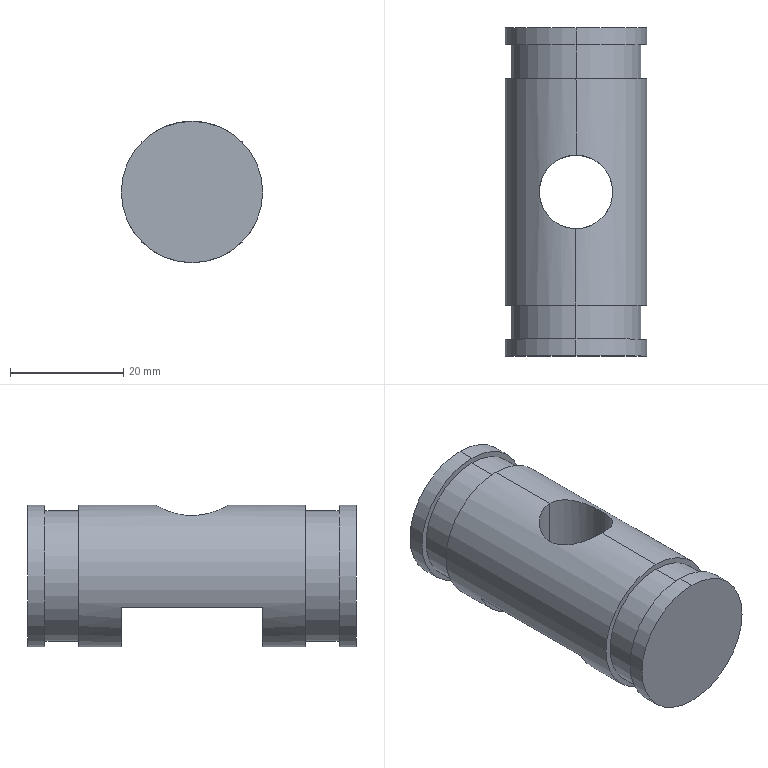Part | SolidWorks | features ICE 3, Extrusion 1, MirrorPattern 1 | 1 solid | 21 faces | box 25 x 58 x 25 mm | volume 22422 mm3 | cylinder 12 | plane 9 | commonest cylinder face diameters 25 x6 23 x4 13 x2
STEP:
#1=CARTESIAN_POINT('',(0.,-6.5,12.5));
#2=VERTEX_POINT('',#1);
#3=CARTESIAN_POINT('',(0.,6.5,12.5));
#4=VERTEX_POINT('',#3);
#5=CARTESIAN_POINT('',(0.,-6.5,12.5));
#6=CARTESIAN_POINT('',(-0.4318,-6.5,12.5));
#7=CARTESIAN_POINT('',(-0.8709,-6.456,12.477));
#8=CARTESIAN_POINT('',(-1.714,-6.285,12.389));
#9=CARTESIAN_POINT('',(-2.124,-6.158,12.325));
#10=CARTESIAN_POINT('',(-2.915,-5.826,12.162));
#11=CARTESIAN_POINT('',(-3.286,-5.624,12.066));
#12=CARTESIAN_POINT('',(-3.982,-5.155,11.854));
#13=CARTESIAN_POINT('',(-4.309,-4.884,11.738));
#14=CARTESIAN_POINT('',(-4.897,-4.294,11.505));
#15=CARTESIAN_POINT('',(-5.161,-3.973,11.388));
#16=CARTESIAN_POINT('',(-5.513,-3.45,11.22));
#17=CARTESIAN_POINT('',(-5.622,-3.269,11.165));
#18=CARTESIAN_POINT('',(-5.822,-2.898,11.062));
#19=CARTESIAN_POINT('',(-5.913,-2.708,11.014));
#20=CARTESIAN_POINT('',(-6.157,-2.126,10.88));
#21=CARTESIAN_POINT('',(-6.283,-1.721,10.807));
#22=CARTESIAN_POINT('',(-6.456,-0.8694,10.704));
#23=CARTESIAN_POINT('',(-6.499,-0.4391,10.677));
#24=CARTESIAN_POINT('',(-6.5,0.2067,10.677));
#25=CARTESIAN_POINT('',(-6.49,0.4224,10.683));
#26=CARTESIAN_POINT('',(-6.447,0.8547,10.709));
#27=CARTESIAN_POINT('',(-6.415,1.071,10.729));
#28=CARTESIAN_POINT('',(-6.287,1.706,10.804));
#29=CARTESIAN_POINT('',(-6.162,2.113,10.877));
#30=CARTESIAN_POINT('',(-5.915,2.704,11.012));
#31=CARTESIAN_POINT('',(-5.823,2.896,11.062));
#32=CARTESIAN_POINT('',(-5.623,3.268,11.164));
#33=CARTESIAN_POINT('',(-5.515,3.447,11.219));
#34=CARTESIAN_POINT('',(-5.282,3.794,11.33));
#35=CARTESIAN_POINT('',(-5.157,3.962,11.388));
#36=CARTESIAN_POINT('',(-4.891,4.287,11.504));
#37=CARTESIAN_POINT('',(-4.749,4.443,11.564));
#38=CARTESIAN_POINT('',(-4.306,4.887,11.739));
#39=CARTESIAN_POINT('',(-3.985,5.152,11.853));
#40=CARTESIAN_POINT('',(-3.289,5.622,12.065));
#41=CARTESIAN_POINT('',(-2.911,5.827,12.163));
#42=CARTESIAN_POINT('',(-2.13,6.156,12.324));
#43=CARTESIAN_POINT('',(-1.724,6.282,12.388));
#44=CARTESIAN_POINT('',(-0.8763,6.455,12.477));
#45=CARTESIAN_POINT('',(-0.4373,6.5,12.5));
#46=CARTESIAN_POINT('',(0.,6.5,12.5));
#47=B_SPLINE_CURVE_WITH_KNOTS('',3,(#5,#6,#7,#8,#9,#10,#11,#12,#13,#14,#15,#16,#17,#18,#19,#20,#21,#22,#23,#24,#25,#26,#27,#28,#29,#30,#31,#32,#33,#34,#35,#36,#37,#38,#39,#40,#41,#42,#43,#44,#45,#46),.UNSPECIFIED.,.F.,.F.,(4,2,2,2,2,2,2,2,2,2,2,2,2,2,2,2,2,2,2,2,4),(0.02071,0.022,0.02329,0.02458,0.02588,0.02717,0.02781,0.02846,0.02975,0.03104,0.03169,0.03233,0.03363,0.03427,0.03492,0.03556,0.03621,0.0375,0.03879,0.04008,0.04138),.UNSPECIFIED.);
#48=EDGE_CURVE('',#2,#4,#47,.T.);
#49=ORIENTED_EDGE('',*,*,#48,.F.);
#50=CARTESIAN_POINT('',(0.,-6.5,-5.5));
#51=VERTEX_POINT('',#50);
#52=CARTESIAN_POINT('',(0.,-6.5,12.5));
#53=DIRECTION('',(0.,0.,-1.));
#54=VECTOR('',#53,1000.);
#55=LINE('',#52,#54);
#56=EDGE_CURVE('',#2,#51,#55,.T.);
#57=ORIENTED_EDGE('',*,*,#56,.T.);
#58=CARTESIAN_POINT('',(0.,6.5,-5.5));
#59=VERTEX_POINT('',#58);
#60=CARTESIAN_POINT('',(0.,0.,-5.5));
#61=DIRECTION('',(0.,0.,-1.));
#62=DIRECTION('',(0.,1.,0.));
#63=AXIS2_PLACEMENT_3D('',#60,#61,#62);
#64=CIRCLE('',#63,6.5);
#65=EDGE_CURVE('',#51,#59,#64,.T.);
#66=ORIENTED_EDGE('',*,*,#65,.T.);
#67=CARTESIAN_POINT('',(0.,6.5,12.5));
#68=DIRECTION('',(0.,0.,-1.));
#69=VECTOR('',#68,1000.);
#70=LINE('',#67,#69);
#71=EDGE_CURVE('',#4,#59,#70,.T.);
#72=ORIENTED_EDGE('',*,*,#71,.F.);
#73=EDGE_LOOP('',(#49,#57,#66,#72));
#74=FACE_OUTER_BOUND('',#73,.T.);
#75=CARTESIAN_POINT('',(0.,0.,12.5));
#76=DIRECTION('',(0.,0.,-1.));
#77=DIRECTION('',(0.,1.,0.));
#78=AXIS2_PLACEMENT_3D('',#75,#76,#77);
#79=CYLINDRICAL_SURFACE('',#78,6.5);
#80=ADVANCED_FACE('',(#74),#79,.F.);
#81=CARTESIAN_POINT('',(0.,-26.,12.5));
#82=VERTEX_POINT('',#81);
#83=CARTESIAN_POINT('',(0.,-26.,-12.5));
#84=VERTEX_POINT('',#83);
#85=CARTESIAN_POINT('',(0.,-26.,0.));
#86=DIRECTION('',(0.,1.,0.));
#87=DIRECTION('',(0.,0.,1.));
#88=AXIS2_PLACEMENT_3D('',#85,#86,#87);
#89=CIRCLE('',#88,12.5);
#90=EDGE_CURVE('',#82,#84,#89,.T.);
#91=ORIENTED_EDGE('',*,*,#90,.F.);
#92=CARTESIAN_POINT('',(0.,-29.,12.5));
#93=VERTEX_POINT('',#92);
#94=CARTESIAN_POINT('',(0.,29.,12.5));
#95=DIRECTION('',(0.,-1.,0.));
#96=VECTOR('',#95,1000.);
#97=LINE('',#94,#96);
#98=EDGE_CURVE('',#82,#93,#97,.T.);
#99=ORIENTED_EDGE('',*,*,#98,.T.);
#100=CARTESIAN_POINT('',(0.,-29.,-12.5));
#101=VERTEX_POINT('',#100);
#102=CARTESIAN_POINT('',(0.,-29.,0.));
#103=DIRECTION('',(0.,1.,0.));
#104=DIRECTION('',(0.,0.,1.));
#105=AXIS2_PLACEMENT_3D('',#102,#103,#104);
#106=CIRCLE('',#105,12.5);
#107=EDGE_CURVE('',#93,#101,#106,.T.);
#108=ORIENTED_EDGE('',*,*,#107,.T.);
#109=CARTESIAN_POINT('',(0.,29.,-12.5));
#110=DIRECTION('',(0.,-1.,0.));
#111=VECTOR('',#110,1000.);
#112=LINE('',#109,#111);
#113=EDGE_CURVE('',#84,#101,#112,.T.);
#114=ORIENTED_EDGE('',*,*,#113,.F.);
#115=EDGE_LOOP('',(#91,#99,#108,#114));
#116=FACE_OUTER_BOUND('',#115,.T.);
#117=CARTESIAN_POINT('',(0.,29.,0.));
#118=DIRECTION('',(0.,-1.,0.));
#119=DIRECTION('',(0.,0.,-1.));
#120=AXIS2_PLACEMENT_3D('',#117,#118,#119);
#121=CYLINDRICAL_SURFACE('',#120,12.5);
#122=ADVANCED_FACE('',(#116),#121,.T.);
#123=CARTESIAN_POINT('',(0.,-20.,11.5));
#124=VERTEX_POINT('',#123);
#125=CARTESIAN_POINT('',(0.,-20.,-11.5));
#126=VERTEX_POINT('',#125);
#127=CARTESIAN_POINT('',(0.,-20.,0.));
#128=DIRECTION('',(0.,1.,0.));
#129=DIRECTION('',(0.,0.,1.));
#130=AXIS2_PLACEMENT_3D('',#127,#128,#129);
#131=CIRCLE('',#130,11.5);
#132=EDGE_CURVE('',#124,#126,#131,.T.);
#133=ORIENTED_EDGE('',*,*,#132,.F.);
#134=CARTESIAN_POINT('',(0.,-26.,11.5));
#135=VERTEX_POINT('',#134);
#136=CARTESIAN_POINT('',(0.,-20.,11.5));
#137=DIRECTION('',(0.,-1.,0.));
#138=VECTOR('',#137,1000.);
#139=LINE('',#136,#138);
#140=EDGE_CURVE('',#124,#135,#139,.T.);
#141=ORIENTED_EDGE('',*,*,#140,.T.);
#142=CARTESIAN_POINT('',(0.,-26.,-11.5));
#143=VERTEX_POINT('',#142);
#144=CARTESIAN_POINT('',(0.,-26.,0.));
#145=DIRECTION('',(0.,1.,0.));
#146=DIRECTION('',(0.,0.,1.));
#147=AXIS2_PLACEMENT_3D('',#144,#145,#146);
#148=CIRCLE('',#147,11.5);
#149=EDGE_CURVE('',#135,#143,#148,.T.);
#150=ORIENTED_EDGE('',*,*,#149,.T.);
#151=CARTESIAN_POINT('',(0.,-20.,-11.5));
#152=DIRECTION('',(0.,-1.,0.));
#153=VECTOR('',#152,1000.);
#154=LINE('',#151,#153);
#155=EDGE_CURVE('',#126,#143,#154,.T.);
#156=ORIENTED_EDGE('',*,*,#155,.F.);
#157=EDGE_LOOP('',(#133,#141,#150,#156));
#158=FACE_OUTER_BOUND('',#157,.T.);
#159=CARTESIAN_POINT('',(0.,-20.,0.));
#160=DIRECTION('',(0.,-1.,0.));
#161=DIRECTION('',(0.,0.,-1.));
#162=AXIS2_PLACEMENT_3D('',#159,#160,#161);
#163=CYLINDRICAL_SURFACE('',#162,11.5);
#164=ADVANCED_FACE('',(#158),#163,.T.);
#165=CARTESIAN_POINT('',(0.,29.,12.5));
#166=VERTEX_POINT('',#165);
#167=CARTESIAN_POINT('',(0.,29.,-12.5));
#168=VERTEX_POINT('',#167);
#169=CARTESIAN_POINT('',(0.,29.,0.));
#170=DIRECTION('',(0.,1.,0.));
#171=DIRECTION('',(0.,0.,1.));
#172=AXIS2_PLACEMENT_3D('',#169,#170,#171);
#173=CIRCLE('',#172,12.5);
#174=EDGE_CURVE('',#166,#168,#173,.T.);
#175=ORIENTED_EDGE('',*,*,#174,.F.);
#176=CARTESIAN_POINT('',(0.,26.,12.5));
#177=VERTEX_POINT('',#176);
#178=CARTESIAN_POINT('',(0.,29.,12.5));
#179=DIRECTION('',(0.,-1.,0.));
#180=VECTOR('',#179,1000.);
#181=LINE('',#178,#180);
#182=EDGE_CURVE('',#166,#177,#181,.T.);
#183=ORIENTED_EDGE('',*,*,#182,.T.);
#184=CARTESIAN_POINT('',(0.,26.,-12.5));
#185=VERTEX_POINT('',#184);
#186=CARTESIAN_POINT('',(0.,26.,0.));
#187=DIRECTION('',(0.,1.,0.));
#188=DIRECTION('',(0.,0.,1.));
#189=AXIS2_PLACEMENT_3D('',#186,#187,#188);
#190=CIRCLE('',#189,12.5);
#191=EDGE_CURVE('',#177,#185,#190,.T.);
#192=ORIENTED_EDGE('',*,*,#191,.T.);
#193=CARTESIAN_POINT('',(0.,29.,-12.5));
#194=DIRECTION('',(0.,-1.,0.));
#195=VECTOR('',#194,1000.);
#196=LINE('',#193,#195);
#197=EDGE_CURVE('',#168,#185,#196,.T.);
#198=ORIENTED_EDGE('',*,*,#197,.F.);
#199=EDGE_LOOP('',(#175,#183,#192,#198));
#200=FACE_OUTER_BOUND('',#199,.T.);
#201=CARTESIAN_POINT('',(0.,29.,0.));
#202=DIRECTION('',(0.,-1.,0.));
#203=DIRECTION('',(0.,0.,-1.));
#204=AXIS2_PLACEMENT_3D('',#201,#202,#203);
#205=CYLINDRICAL_SURFACE('',#204,12.5);
#206=ADVANCED_FACE('',(#200),#205,.T.);
#207=CARTESIAN_POINT('',(0.,20.,11.5));
#208=VERTEX_POINT('',#207);
#209=CARTESIAN_POINT('',(0.,20.,-11.5));
#210=VERTEX_POINT('',#209);
#211=CARTESIAN_POINT('',(0.,20.,0.));
#212=DIRECTION('',(0.,1.,0.));
#213=DIRECTION('',(0.,0.,1.));
#214=AXIS2_PLACEMENT_3D('',#211,#212,#213);
#215=CIRCLE('',#214,11.5);
#216=EDGE_CURVE('',#208,#210,#215,.T.);
#217=ORIENTED_EDGE('',*,*,#216,.T.);
#218=CARTESIAN_POINT('',(0.,26.,-11.5));
#219=VERTEX_POINT('',#218);
#220=CARTESIAN_POINT('',(0.,20.,-11.5));
#221=DIRECTION('',(0.,1.,0.));
#222=VECTOR('',#221,1000.);
#223=LINE('',#220,#222);
#224=EDGE_CURVE('',#210,#219,#223,.T.);
#225=ORIENTED_EDGE('',*,*,#224,.T.);
#226=CARTESIAN_POINT('',(0.,26.,11.5));
#227=VERTEX_POINT('',#226);
#228=CARTESIAN_POINT('',(0.,26.,0.));
#229=DIRECTION('',(0.,1.,0.));
#230=DIRECTION('',(0.,0.,1.));
#231=AXIS2_PLACEMENT_3D('',#228,#229,#230);
#232=CIRCLE('',#231,11.5);
#233=EDGE_CURVE('',#227,#219,#232,.T.);
#234=ORIENTED_EDGE('',*,*,#233,.F.);
#235=CARTESIAN_POINT('',(0.,20.,11.5));
#236=DIRECTION('',(0.,1.,0.));
#237=VECTOR('',#236,1000.);
#238=LINE('',#235,#237);
#239=EDGE_CURVE('',#208,#227,#238,.T.);
#240=ORIENTED_EDGE('',*,*,#239,.F.);
#241=EDGE_LOOP('',(#217,#225,#234,#240));
#242=FACE_OUTER_BOUND('',#241,.T.);
#243=CARTESIAN_POINT('',(0.,20.,0.));
#244=DIRECTION('',(0.,1.,0.));
#245=DIRECTION('',(0.,0.,1.));
#246=AXIS2_PLACEMENT_3D('',#243,#244,#245);
#247=CYLINDRICAL_SURFACE('',#246,11.5);
#248=ADVANCED_FACE('',(#242),#247,.T.);
#249=CARTESIAN_POINT('',(0.,20.,12.5));
#250=VERTEX_POINT('',#249);
#251=CARTESIAN_POINT('',(0.,20.,-12.5));
#252=VERTEX_POINT('',#251);
#253=CARTESIAN_POINT('',(0.,20.,0.));
#254=DIRECTION('',(0.,1.,0.));
#255=DIRECTION('',(0.,0.,1.));
#256=AXIS2_PLACEMENT_3D('',#253,#254,#255);
#257=CIRCLE('',#256,12.5);
#258=EDGE_CURVE('',#250,#252,#257,.T.);
#259=ORIENTED_EDGE('',*,*,#258,.F.);
#260=CARTESIAN_POINT('',(0.,29.,12.5));
#261=DIRECTION('',(0.,-1.,0.));
#262=VECTOR('',#261,1000.);
#263=LINE('',#260,#262);
#264=EDGE_CURVE('',#250,#4,#263,.T.);
#265=ORIENTED_EDGE('',*,*,#264,.T.);
#266=CARTESIAN_POINT('',(0.,6.5,12.5));
#267=CARTESIAN_POINT('',(0.4382,6.5,12.5));
#268=CARTESIAN_POINT('',(0.8676,6.456,12.477));
#269=CARTESIAN_POINT('',(1.71,6.286,12.39));
#270=CARTESIAN_POINT('',(2.127,6.157,12.324));
#271=CARTESIAN_POINT('',(2.912,5.827,12.163));
#272=CARTESIAN_POINT('',(3.283,5.626,12.067));
#273=CARTESIAN_POINT('',(3.809,5.272,11.907));
#274=CARTESIAN_POINT('',(3.978,5.145,11.851));
#275=CARTESIAN_POINT('',(4.301,4.878,11.738));
#276=CARTESIAN_POINT('',(4.455,4.738,11.68));
#277=CARTESIAN_POINT('',(4.749,4.443,11.564));
#278=CARTESIAN_POINT('',(4.889,4.289,11.505));
#279=CARTESIAN_POINT('',(5.155,3.965,11.389));
#280=CARTESIAN_POINT('',(5.281,3.796,11.33));
#281=CARTESIAN_POINT('',(5.632,3.272,11.162));
#282=CARTESIAN_POINT('',(5.83,2.904,11.058));
#283=CARTESIAN_POINT('',(6.075,2.32,10.925));
#284=CARTESIAN_POINT('',(6.148,2.121,10.884));
#285=CARTESIAN_POINT('',(6.275,1.709,10.811));
#286=CARTESIAN_POINT('',(6.328,1.499,10.78));
#287=CARTESIAN_POINT('',(6.456,0.8676,10.704));
#288=CARTESIAN_POINT('',(6.5,0.4405,10.677));
#289=CARTESIAN_POINT('',(6.5,-0.2097,10.677));
#290=CARTESIAN_POINT('',(6.489,-0.4295,10.684));
#291=CARTESIAN_POINT('',(6.446,-0.8623,10.71));
#292=CARTESIAN_POINT('',(6.414,-1.076,10.729));
#293=CARTESIAN_POINT('',(6.329,-1.497,10.779));
#294=CARTESIAN_POINT('',(6.276,-1.704,10.81));
#295=CARTESIAN_POINT('',(6.15,-2.114,10.883));
#296=CARTESIAN_POINT('',(6.077,-2.317,10.924));
#297=CARTESIAN_POINT('',(5.829,-2.907,11.059));
#298=CARTESIAN_POINT('',(5.63,-3.276,11.164));
#299=CARTESIAN_POINT('',(5.278,-3.8,11.332));
#300=CARTESIAN_POINT('',(5.151,-3.97,11.39));
#301=CARTESIAN_POINT('',(4.885,-4.293,11.507));
#302=CARTESIAN_POINT('',(4.745,-4.448,11.566));
#303=CARTESIAN_POINT('',(4.303,-4.889,11.74));
#304=CARTESIAN_POINT('',(3.981,-5.156,11.855));
#305=CARTESIAN_POINT('',(3.277,-5.63,12.069));
#306=CARTESIAN_POINT('',(2.906,-5.83,12.164));
#307=CARTESIAN_POINT('',(2.32,-6.075,12.284));
#308=CARTESIAN_POINT('',(2.12,-6.148,12.321));
#309=CARTESIAN_POINT('',(1.71,-6.275,12.384));
#310=CARTESIAN_POINT('',(1.498,-6.329,12.412));
#311=CARTESIAN_POINT('',(0.8613,-6.457,12.478));
#312=CARTESIAN_POINT('',(0.4326,-6.5,12.5));
#313=CARTESIAN_POINT('',(0.,-6.5,12.5));
#314=B_SPLINE_CURVE_WITH_KNOTS('',3,(#266,#267,#268,#269,#270,#271,#272,#273,#274,#275,#276,#277,#278,#279,#280,#281,#282,#283,#284,#285,#286,#287,#288,#289,#290,#291,#292,#293,#294,#295,#296,#297,#298,#299,#300,#301,#302,#303,#304,#305,#306,#307,#308,#309,#310,#311,#312,#313),.UNSPECIFIED.,.F.,.F.,(4,2,2,2,2,2,2,2,2,2,2,2,2,2,2,2,2,2,2,2,2,2,2,4),(0.,0.001294,0.002589,0.003883,0.00453,0.005177,0.005824,0.006472,0.007766,0.008413,0.00906,0.01035,0.011,0.01165,0.0123,0.01294,0.01424,0.01488,0.01553,0.01683,0.01812,0.01877,0.01941,0.02071),.UNSPECIFIED.);
#315=EDGE_CURVE('',#4,#2,#314,.T.);
#316=ORIENTED_EDGE('',*,*,#315,.T.);
#317=CARTESIAN_POINT('',(0.,-20.,12.5));
#318=VERTEX_POINT('',#317);
#319=CARTESIAN_POINT('',(0.,29.,12.5));
#320=DIRECTION('',(0.,-1.,0.));
#321=VECTOR('',#320,1000.);
#322=LINE('',#319,#321);
#323=EDGE_CURVE('',#2,#318,#322,.T.);
#324=ORIENTED_EDGE('',*,*,#323,.T.);
#325=CARTESIAN_POINT('',(0.,-20.,-12.5));
#326=VERTEX_POINT('',#325);
#327=CARTESIAN_POINT('',(0.,-20.,0.));
#328=DIRECTION('',(0.,1.,0.));
#329=DIRECTION('',(0.,0.,1.));
#330=AXIS2_PLACEMENT_3D('',#327,#328,#329);
#331=CIRCLE('',#330,12.5);
#332=EDGE_CURVE('',#318,#326,#331,.T.);
#333=ORIENTED_EDGE('',*,*,#332,.T.);
#334=CARTESIAN_POINT('',(0.,-12.5,-12.5));
#335=VERTEX_POINT('',#334);
#336=CARTESIAN_POINT('',(0.,29.,-12.5));
#337=DIRECTION('',(0.,-1.,0.));
#338=VECTOR('',#337,1000.);
#339=LINE('',#336,#338);
#340=EDGE_CURVE('',#335,#326,#339,.T.);
#341=ORIENTED_EDGE('',*,*,#340,.F.);
#342=CARTESIAN_POINT('',(11.225,-12.5,-5.5));
#343=VERTEX_POINT('',#342);
#344=CARTESIAN_POINT('',(0.,-12.5,0.));
#345=DIRECTION('',(0.,-1.,0.));
#346=DIRECTION('',(0.,0.,-1.));
#347=AXIS2_PLACEMENT_3D('',#344,#345,#346);
#348=CIRCLE('',#347,12.5);
#349=EDGE_CURVE('',#335,#343,#348,.T.);
#350=ORIENTED_EDGE('',*,*,#349,.T.);
#351=CARTESIAN_POINT('',(11.225,12.5,-5.5));
#352=VERTEX_POINT('',#351);
#353=CARTESIAN_POINT('',(11.225,29.,-5.5));
#354=DIRECTION('',(0.,1.,0.));
#355=VECTOR('',#354,1000.);
#356=LINE('',#353,#355);
#357=EDGE_CURVE('',#343,#352,#356,.T.);
#358=ORIENTED_EDGE('',*,*,#357,.T.);
#359=CARTESIAN_POINT('',(0.,12.5,-12.5));
#360=VERTEX_POINT('',#359);
#361=CARTESIAN_POINT('',(0.,12.5,0.));
#362=DIRECTION('',(0.,1.,0.));
#363=DIRECTION('',(0.,0.,1.));
#364=AXIS2_PLACEMENT_3D('',#361,#362,#363);
#365=CIRCLE('',#364,12.5);
#366=EDGE_CURVE('',#352,#360,#365,.T.);
#367=ORIENTED_EDGE('',*,*,#366,.T.);
#368=CARTESIAN_POINT('',(0.,29.,-12.5));
#369=DIRECTION('',(0.,-1.,0.));
#370=VECTOR('',#369,1000.);
#371=LINE('',#368,#370);
#372=EDGE_CURVE('',#252,#360,#371,.T.);
#373=ORIENTED_EDGE('',*,*,#372,.F.);
#374=EDGE_LOOP('',(#259,#265,#316,#324,#333,#341,#350,#358,#367,#373));
#375=FACE_OUTER_BOUND('',#374,.T.);
#376=CARTESIAN_POINT('',(0.,29.,0.));
#377=DIRECTION('',(0.,-1.,0.));
#378=DIRECTION('',(0.,0.,-1.));
#379=AXIS2_PLACEMENT_3D('',#376,#377,#378);
#380=CYLINDRICAL_SURFACE('',#379,12.5);
#381=ADVANCED_FACE('',(#375),#380,.T.);
#382=ORIENTED_EDGE('',*,*,#264,.F.);
#383=CARTESIAN_POINT('',(0.,20.,0.));
#384=DIRECTION('',(0.,1.,0.));
#385=DIRECTION('',(0.,0.,1.));
#386=AXIS2_PLACEMENT_3D('',#383,#384,#385);
#387=CIRCLE('',#386,12.5);
#388=EDGE_CURVE('',#252,#250,#387,.T.);
#389=ORIENTED_EDGE('',*,*,#388,.F.);
#390=ORIENTED_EDGE('',*,*,#372,.T.);
#391=CARTESIAN_POINT('',(-11.225,12.5,-5.5));
#392=VERTEX_POINT('',#391);
#393=CARTESIAN_POINT('',(0.,12.5,0.));
#394=DIRECTION('',(0.,1.,0.));
#395=DIRECTION('',(0.,0.,1.));
#396=AXIS2_PLACEMENT_3D('',#393,#394,#395);
#397=CIRCLE('',#396,12.5);
#398=EDGE_CURVE('',#360,#392,#397,.T.);
#399=ORIENTED_EDGE('',*,*,#398,.T.);
#400=CARTESIAN_POINT('',(-11.225,-12.5,-5.5));
#401=VERTEX_POINT('',#400);
#402=CARTESIAN_POINT('',(-11.225,29.,-5.5));
#403=DIRECTION('',(0.,-1.,0.));
#404=VECTOR('',#403,1000.);
#405=LINE('',#402,#404);
#406=EDGE_CURVE('',#392,#401,#405,.T.);
#407=ORIENTED_EDGE('',*,*,#406,.T.);
#408=CARTESIAN_POINT('',(0.,-12.5,0.));
#409=DIRECTION('',(0.,-1.,0.));
#410=DIRECTION('',(0.,0.,-1.));
#411=AXIS2_PLACEMENT_3D('',#408,#409,#410);
#412=CIRCLE('',#411,12.5);
#413=EDGE_CURVE('',#401,#335,#412,.T.);
#414=ORIENTED_EDGE('',*,*,#413,.T.);
#415=ORIENTED_EDGE('',*,*,#340,.T.);
#416=CARTESIAN_POINT('',(0.,-20.,0.));
#417=DIRECTION('',(0.,1.,0.));
#418=DIRECTION('',(0.,0.,1.));
#419=AXIS2_PLACEMENT_3D('',#416,#417,#418);
#420=CIRCLE('',#419,12.5);
#421=EDGE_CURVE('',#326,#318,#420,.T.);
#422=ORIENTED_EDGE('',*,*,#421,.T.);
#423=ORIENTED_EDGE('',*,*,#323,.F.);
#424=ORIENTED_EDGE('',*,*,#48,.T.);
#425=EDGE_LOOP('',(#382,#389,#390,#399,#407,#414,#415,#422,#423,#424));
#426=FACE_OUTER_BOUND('',#425,.T.);
#427=CARTESIAN_POINT('',(0.,29.,0.));
#428=DIRECTION('',(0.,-1.,0.));
#429=DIRECTION('',(0.,0.,-1.));
#430=AXIS2_PLACEMENT_3D('',#427,#428,#429);
#431=CYLINDRICAL_SURFACE('',#430,12.5);
#432=ADVANCED_FACE('',(#426),#431,.T.);
#433=ORIENTED_EDGE('',*,*,#216,.F.);
#434=CARTESIAN_POINT('',(0.,20.,0.));
#435=DIRECTION('',(0.,1.,0.));
#436=DIRECTION('',(0.,0.,1.));
#437=AXIS2_PLACEMENT_3D('',#434,#435,#436);
#438=CIRCLE('',#437,11.5);
#439=EDGE_CURVE('',#210,#208,#438,.T.);
#440=ORIENTED_EDGE('',*,*,#439,.F.);
#441=EDGE_LOOP('',(#433,#440));
#442=FACE_BOUND('',#441,.T.);
#443=ORIENTED_EDGE('',*,*,#388,.T.);
#444=ORIENTED_EDGE('',*,*,#258,.T.);
#445=EDGE_LOOP('',(#443,#444));
#446=FACE_OUTER_BOUND('',#445,.T.);
#447=CARTESIAN_POINT('',(0.,20.,0.));
#448=DIRECTION('',(0.,1.,0.));
#449=DIRECTION('',(0.,0.,1.));
#450=AXIS2_PLACEMENT_3D('',#447,#448,#449);
#451=PLANE('',#450);
#452=ADVANCED_FACE('',(#442,#446),#451,.T.);
#453=ORIENTED_EDGE('',*,*,#233,.T.);
#454=CARTESIAN_POINT('',(0.,26.,0.));
#455=DIRECTION('',(0.,1.,0.));
#456=DIRECTION('',(0.,0.,1.));
#457=AXIS2_PLACEMENT_3D('',#454,#455,#456);
#458=CIRCLE('',#457,11.5);
#459=EDGE_CURVE('',#219,#227,#458,.T.);
#460=ORIENTED_EDGE('',*,*,#459,.T.);
#461=EDGE_LOOP('',(#453,#460));
#462=FACE_BOUND('',#461,.T.);
#463=CARTESIAN_POINT('',(0.,26.,0.));
#464=DIRECTION('',(0.,1.,0.));
#465=DIRECTION('',(0.,0.,1.));
#466=AXIS2_PLACEMENT_3D('',#463,#464,#465);
#467=CIRCLE('',#466,12.5);
#468=EDGE_CURVE('',#185,#177,#467,.T.);
#469=ORIENTED_EDGE('',*,*,#468,.F.);
#470=ORIENTED_EDGE('',*,*,#191,.F.);
#471=EDGE_LOOP('',(#469,#470));
#472=FACE_OUTER_BOUND('',#471,.T.);
#473=CARTESIAN_POINT('',(0.,26.,0.));
#474=DIRECTION('',(0.,1.,0.));
#475=DIRECTION('',(0.,0.,1.));
#476=AXIS2_PLACEMENT_3D('',#473,#474,#475);
#477=PLANE('',#476);
#478=ADVANCED_FACE('',(#462,#472),#477,.F.);
#479=ORIENTED_EDGE('',*,*,#224,.F.);
#480=ORIENTED_EDGE('',*,*,#439,.T.);
#481=ORIENTED_EDGE('',*,*,#239,.T.);
#482=ORIENTED_EDGE('',*,*,#459,.F.);
#483=EDGE_LOOP('',(#479,#480,#481,#482));
#484=FACE_OUTER_BOUND('',#483,.T.);
#485=CARTESIAN_POINT('',(0.,20.,0.));
#486=DIRECTION('',(0.,1.,0.));
#487=DIRECTION('',(0.,0.,1.));
#488=AXIS2_PLACEMENT_3D('',#485,#486,#487);
#489=CYLINDRICAL_SURFACE('',#488,11.5);
#490=ADVANCED_FACE('',(#484),#489,.T.);
#491=CARTESIAN_POINT('',(0.,29.,0.));
#492=DIRECTION('',(0.,1.,0.));
#493=DIRECTION('',(0.,0.,1.));
#494=AXIS2_PLACEMENT_3D('',#491,#492,#493);
#495=CIRCLE('',#494,12.5);
#496=EDGE_CURVE('',#168,#166,#495,.T.);
#497=ORIENTED_EDGE('',*,*,#496,.T.);
#498=ORIENTED_EDGE('',*,*,#174,.T.);
#499=EDGE_LOOP('',(#497,#498));
#500=FACE_OUTER_BOUND('',#499,.T.);
#501=CARTESIAN_POINT('',(0.,29.,0.));
#502=DIRECTION('',(0.,1.,0.));
#503=DIRECTION('',(0.,0.,1.));
#504=AXIS2_PLACEMENT_3D('',#501,#502,#503);
#505=PLANE('',#504);
#506=ADVANCED_FACE('',(#500),#505,.T.);
#507=ORIENTED_EDGE('',*,*,#182,.F.);
#508=ORIENTED_EDGE('',*,*,#496,.F.);
#509=ORIENTED_EDGE('',*,*,#197,.T.);
#510=ORIENTED_EDGE('',*,*,#468,.T.);
#511=EDGE_LOOP('',(#507,#508,#509,#510));
#512=FACE_OUTER_BOUND('',#511,.T.);
#513=CARTESIAN_POINT('',(0.,29.,0.));
#514=DIRECTION('',(0.,-1.,0.));
#515=DIRECTION('',(0.,0.,-1.));
#516=AXIS2_PLACEMENT_3D('',#513,#514,#515);
#517=CYLINDRICAL_SURFACE('',#516,12.5);
#518=ADVANCED_FACE('',(#512),#517,.T.);
#519=ORIENTED_EDGE('',*,*,#421,.F.);
#520=ORIENTED_EDGE('',*,*,#332,.F.);
#521=EDGE_LOOP('',(#519,#520));
#522=FACE_OUTER_BOUND('',#521,.T.);
#523=CARTESIAN_POINT('',(0.,-20.,0.));
#524=DIRECTION('',(0.,1.,0.));
#525=DIRECTION('',(0.,0.,1.));
#526=AXIS2_PLACEMENT_3D('',#523,#524,#525);
#527=CIRCLE('',#526,11.5);
#528=EDGE_CURVE('',#126,#124,#527,.T.);
#529=ORIENTED_EDGE('',*,*,#528,.T.);
#530=ORIENTED_EDGE('',*,*,#132,.T.);
#531=EDGE_LOOP('',(#529,#530));
#532=FACE_BOUND('',#531,.T.);
#533=CARTESIAN_POINT('',(0.,-20.,0.));
#534=DIRECTION('',(0.,-1.,0.));
#535=DIRECTION('',(0.,0.,1.));
#536=AXIS2_PLACEMENT_3D('',#533,#534,#535);
#537=PLANE('',#536);
#538=ADVANCED_FACE('',(#522,#532),#537,.T.);
#539=CARTESIAN_POINT('',(0.,-26.,0.));
#540=DIRECTION('',(0.,1.,0.));
#541=DIRECTION('',(0.,0.,1.));
#542=AXIS2_PLACEMENT_3D('',#539,#540,#541);
#543=CIRCLE('',#542,12.5);
#544=EDGE_CURVE('',#84,#82,#543,.T.);
#545=ORIENTED_EDGE('',*,*,#544,.T.);
#546=ORIENTED_EDGE('',*,*,#90,.T.);
#547=EDGE_LOOP('',(#545,#546));
#548=FACE_OUTER_BOUND('',#547,.T.);
#549=CARTESIAN_POINT('',(0.,-26.,0.));
#550=DIRECTION('',(0.,1.,0.));
#551=DIRECTION('',(0.,0.,1.));
#552=AXIS2_PLACEMENT_3D('',#549,#550,#551);
#553=CIRCLE('',#552,11.5);
#554=EDGE_CURVE('',#143,#135,#553,.T.);
#555=ORIENTED_EDGE('',*,*,#554,.F.);
#556=ORIENTED_EDGE('',*,*,#149,.F.);
#557=EDGE_LOOP('',(#555,#556));
#558=FACE_BOUND('',#557,.T.);
#559=CARTESIAN_POINT('',(0.,-26.,0.));
#560=DIRECTION('',(0.,-1.,0.));
#561=DIRECTION('',(0.,0.,1.));
#562=AXIS2_PLACEMENT_3D('',#559,#560,#561);
#563=PLANE('',#562);
#564=ADVANCED_FACE('',(#548,#558),#563,.F.);
#565=ORIENTED_EDGE('',*,*,#140,.F.);
#566=ORIENTED_EDGE('',*,*,#528,.F.);
#567=ORIENTED_EDGE('',*,*,#155,.T.);
#568=ORIENTED_EDGE('',*,*,#554,.T.);
#569=EDGE_LOOP('',(#565,#566,#567,#568));
#570=FACE_OUTER_BOUND('',#569,.T.);
#571=CARTESIAN_POINT('',(0.,-20.,0.));
#572=DIRECTION('',(0.,-1.,0.));
#573=DIRECTION('',(0.,0.,-1.));
#574=AXIS2_PLACEMENT_3D('',#571,#572,#573);
#575=CYLINDRICAL_SURFACE('',#574,11.5);
#576=ADVANCED_FACE('',(#570),#575,.T.);
#577=CARTESIAN_POINT('',(0.,-29.,0.));
#578=DIRECTION('',(0.,1.,0.));
#579=DIRECTION('',(0.,0.,1.));
#580=AXIS2_PLACEMENT_3D('',#577,#578,#579);
#581=CIRCLE('',#580,12.5);
#582=EDGE_CURVE('',#101,#93,#581,.T.);
#583=ORIENTED_EDGE('',*,*,#582,.F.);
#584=ORIENTED_EDGE('',*,*,#107,.F.);
#585=EDGE_LOOP('',(#583,#584));
#586=FACE_OUTER_BOUND('',#585,.T.);
#587=CARTESIAN_POINT('',(0.,-29.,0.));
#588=DIRECTION('',(0.,1.,0.));
#589=DIRECTION('',(0.,0.,1.));
#590=AXIS2_PLACEMENT_3D('',#587,#588,#589);
#591=PLANE('',#590);
#592=ADVANCED_FACE('',(#586),#591,.F.);
#593=ORIENTED_EDGE('',*,*,#98,.F.);
#594=ORIENTED_EDGE('',*,*,#544,.F.);
#595=ORIENTED_EDGE('',*,*,#113,.T.);
#596=ORIENTED_EDGE('',*,*,#582,.T.);
#597=EDGE_LOOP('',(#593,#594,#595,#596));
#598=FACE_OUTER_BOUND('',#597,.T.);
#599=CARTESIAN_POINT('',(0.,29.,0.));
#600=DIRECTION('',(0.,-1.,0.));
#601=DIRECTION('',(0.,0.,-1.));
#602=AXIS2_PLACEMENT_3D('',#599,#600,#601);
#603=CYLINDRICAL_SURFACE('',#602,12.5);
#604=ADVANCED_FACE('',(#598),#603,.T.);
#605=ORIENTED_EDGE('',*,*,#413,.F.);
#606=CARTESIAN_POINT('',(-33.,-12.5,-5.5));
#607=DIRECTION('',(1.,0.,0.));
#608=VECTOR('',#607,1000.);
#609=LINE('',#606,#608);
#610=EDGE_CURVE('',#401,#343,#609,.T.);
#611=ORIENTED_EDGE('',*,*,#610,.T.);
#612=ORIENTED_EDGE('',*,*,#349,.F.);
#613=EDGE_LOOP('',(#605,#611,#612));
#614=FACE_OUTER_BOUND('',#613,.T.);
#615=CARTESIAN_POINT('',(-33.,-12.5,-12.5));
#616=DIRECTION('',(0.,-1.,0.));
#617=DIRECTION('',(0.,0.,-1.));
#618=AXIS2_PLACEMENT_3D('',#615,#616,#617);
#619=PLANE('',#618);
#620=ADVANCED_FACE('',(#614),#619,.F.);
#621=CARTESIAN_POINT('',(0.,0.,-5.5));
#622=DIRECTION('',(0.,0.,-1.));
#623=DIRECTION('',(0.,1.,0.));
#624=AXIS2_PLACEMENT_3D('',#621,#622,#623);
#625=CIRCLE('',#624,6.5);
#626=EDGE_CURVE('',#59,#51,#625,.T.);
#627=ORIENTED_EDGE('',*,*,#626,.F.);
#628=ORIENTED_EDGE('',*,*,#65,.F.);
#629=EDGE_LOOP('',(#627,#628));
#630=FACE_BOUND('',#629,.T.);
#631=CARTESIAN_POINT('',(-33.,12.5,-5.5));
#632=DIRECTION('',(1.,0.,0.));
#633=VECTOR('',#632,1000.);
#634=LINE('',#631,#633);
#635=EDGE_CURVE('',#392,#352,#634,.T.);
#636=ORIENTED_EDGE('',*,*,#635,.T.);
#637=ORIENTED_EDGE('',*,*,#357,.F.);
#638=ORIENTED_EDGE('',*,*,#610,.F.);
#639=ORIENTED_EDGE('',*,*,#406,.F.);
#640=EDGE_LOOP('',(#636,#637,#638,#639));
#641=FACE_OUTER_BOUND('',#640,.T.);
#642=CARTESIAN_POINT('',(-33.,12.5,-5.5));
#643=DIRECTION('',(0.,0.,1.));
#644=DIRECTION('',(0.,-1.,0.));
#645=AXIS2_PLACEMENT_3D('',#642,#643,#644);
#646=PLANE('',#645);
#647=ADVANCED_FACE('',(#630,#641),#646,.F.);
#648=ORIENTED_EDGE('',*,*,#635,.F.);
#649=ORIENTED_EDGE('',*,*,#398,.F.);
#650=ORIENTED_EDGE('',*,*,#366,.F.);
#651=EDGE_LOOP('',(#648,#649,#650));
#652=FACE_OUTER_BOUND('',#651,.T.);
#653=CARTESIAN_POINT('',(-33.,12.5,-12.5));
#654=DIRECTION('',(0.,1.,0.));
#655=DIRECTION('',(0.,0.,1.));
#656=AXIS2_PLACEMENT_3D('',#653,#654,#655);
#657=PLANE('',#656);
#658=ADVANCED_FACE('',(#652),#657,.F.);
#659=ORIENTED_EDGE('',*,*,#56,.F.);
#660=ORIENTED_EDGE('',*,*,#315,.F.);
#661=ORIENTED_EDGE('',*,*,#71,.T.);
#662=ORIENTED_EDGE('',*,*,#626,.T.);
#663=EDGE_LOOP('',(#659,#660,#661,#662));
#664=FACE_OUTER_BOUND('',#663,.T.);
#665=CARTESIAN_POINT('',(0.,0.,12.5));
#666=DIRECTION('',(0.,0.,-1.));
#667=DIRECTION('',(0.,1.,0.));
#668=AXIS2_PLACEMENT_3D('',#665,#666,#667);
#669=CYLINDRICAL_SURFACE('',#668,6.5);
#670=ADVANCED_FACE('',(#664),#669,.F.);
#671=CLOSED_SHELL('',(#80,#122,#164,#206,#248,#381,#432,#452,#478,#490,#506,#518,#538,#564,#576,#592,#604,#620,#647,#658,#670));
#672=MANIFOLD_SOLID_BREP('',#671);
#673=CARTESIAN_POINT('',(0.,0.,0.));
#674=DIRECTION('',(0.,0.,1.));
#675=DIRECTION('',(1.,0.,0.));
#676=AXIS2_PLACEMENT_3D('',#673,#674,#675);
#677=(LENGTH_UNIT()NAMED_UNIT(*)SI_UNIT(.MILLI.,.METRE.));
#678=UNCERTAINTY_MEASURE_WITH_UNIT(LENGTH_MEASURE(0.00001),#677,'','');
#679=(NAMED_UNIT(*)PLANE_ANGLE_UNIT()SI_UNIT($,.RADIAN.));
#680=(NAMED_UNIT(*)SI_UNIT($,.STERADIAN.)SOLID_ANGLE_UNIT());
#681=(GEOMETRIC_REPRESENTATION_CONTEXT(3)GLOBAL_UNCERTAINTY_ASSIGNED_CONTEXT((#678))GLOBAL_UNIT_ASSIGNED_CONTEXT((#677,#679,#680))REPRESENTATION_CONTEXT('',''));
#682=ADVANCED_BREP_SHAPE_REPRESENTATION('',(#672,#676),#681);